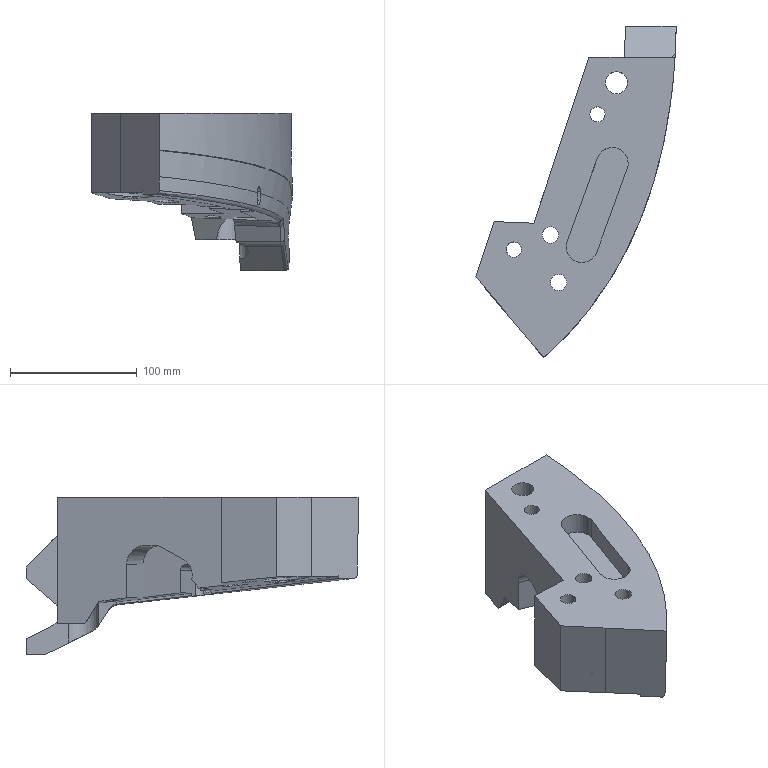Part | NX | features solid 2 | 1 solid | 95 faces | box 158.277 x 262.268 x 124.337 mm | volume 1253108 mm3 | plane 36 | spline 34 | cylinder 22 | sphere 2 | cone 1 | commonest cylinder face diameters 10 x5 20 x4 7.1 x2 12 x2 13 x2 25 x2